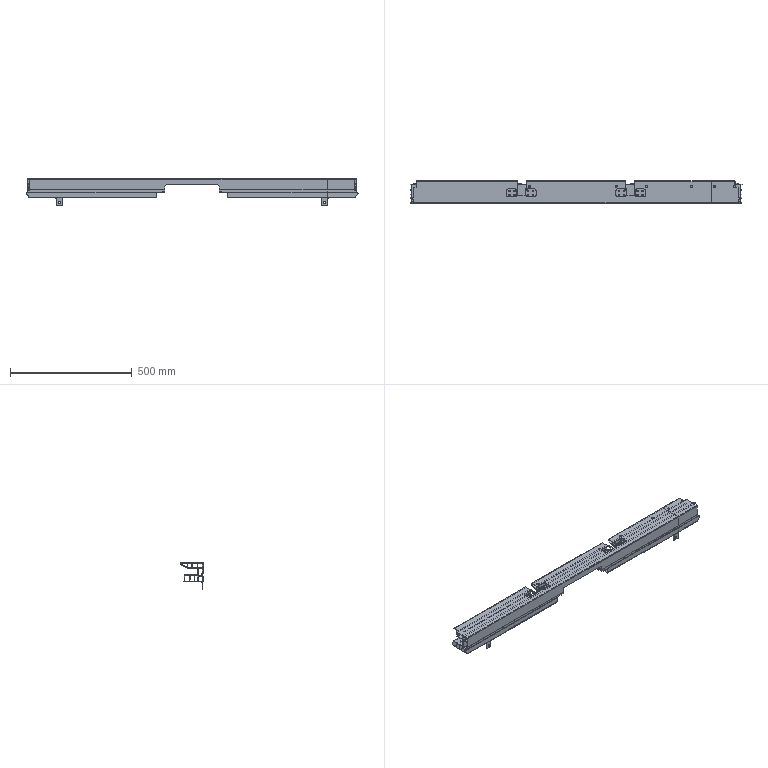NC program | NX | posted with a generic post | part box 1365 x 90.95 x 108.501 mm
Lines 6615 to 7500 of 25066:
(CAVITY_MILL_COPY , TOOL : D10)
N13216 T10 M6
N13218 G54
N13220 G17 G0 G90 X-676.615 Y32.745 B0. C0. S6500 M3
N13222 G43 Z30. H10
N13224 Z0.508
N13226 G94 G1 Z-0.992 F1000.
N13228 X-675.092 Y31.92
N13230 G3 X-674.092 Y31.947 R1.
N13232 G1 X-672.75 Y32.772 F1800.
N13234 Y34.347
N13236 G3 X-673.25 Y35.213 R1.
N13238 G1 X-674.75 Y36.079
N13240 Z0.508
N13242 G0 X-676.615 Y32.745 Z-0.482
N13244 G1 Z-1.982 F1000.
N13246 X-675.092 Y31.92
N13248 G3 X-674.092 Y31.947 R1.
N13250 G1 X-672.75 Y32.772 F1800.
N13252 Y34.347
N13254 G3 X-673.25 Y35.213 R1.
N13256 G1 X-674.75 Y36.079
N13258 Z-0.482
N13260 G0 X-676.615 Y32.745 Z-1.473
N13262 G1 Z-2.973 F1000.
N13264 X-675.092 Y31.92
N13266 G3 X-674.092 Y31.947 R1.
N13268 G1 X-672.75 Y32.772 F1800.
N13270 Y34.347
N13272 G3 X-673.25 Y35.213 R1.
N13274 G1 X-674.75 Y36.079
N13276 Z-1.473
N13278 G0 X-676.615 Y32.745 Z-2.463
N13280 G1 Z-3.963 F1000.
N13282 X-675.092 Y31.92
N13284 G3 X-674.092 Y31.947 R1.
N13286 G1 X-672.75 Y32.772 F1800.
N13288 Y34.347
N13290 G3 X-673.25 Y35.213 R1.
N13292 G1 X-674.75 Y36.079
N13294 Z-2.463
N13296 G0 X-676.615 Y32.745 Z-3.454
N13298 G1 Z-4.954 F1000.
N13300 X-675.092 Y31.92
N13302 G3 X-674.092 Y31.947 R1.
N13304 G1 X-672.75 Y32.772 F1800.
N13306 Y34.347
N13308 G3 X-673.25 Y35.213 R1.
N13310 G1 X-674.75 Y36.079
N13312 Z-3.454
N13314 G0 X-676.615 Y32.745 Z-4.444
N13316 G1 Z-5.944 F1000.
N13318 X-675.092 Y31.92
N13320 G3 X-674.092 Y31.947 R1.
N13322 G1 X-672.75 Y32.772 F1800.
N13324 Y34.347
N13326 G3 X-673.25 Y35.213 R1.
N13328 G1 X-674.75 Y36.079
N13330 Z-4.444
N13332 G0 X-676.615 Y32.745 Z-5.435
N13334 G1 Z-6.935 F1000.
N13336 X-675.092 Y31.92
N13338 G3 X-674.092 Y31.947 R1.
N13340 G1 X-672.75 Y32.772 F1800.
N13342 Y34.347
N13344 G3 X-673.25 Y35.213 R1.
N13346 G1 X-674.75 Y36.079
N13348 Z-5.435
N13350 G0 X-676.615 Y32.745 Z-6.425
N13352 G1 Z-7.925 F1000.
N13354 X-675.092 Y31.92
N13356 G3 X-674.092 Y31.947 R1.
N13358 G1 X-672.75 Y32.772 F1800.
N13360 Y34.347
N13362 G3 X-673.25 Y35.213 R1.
N13364 G1 X-674.75 Y36.079
N13366 Z-6.425
N13368 G0 X-676.615 Y32.745 Z-7.416
N13370 G1 Z-8.916 F1000.
N13372 X-675.092 Y31.92
N13374 G3 X-674.092 Y31.947 R1.
N13376 G1 X-672.75 Y32.772 F1800.
N13378 Y34.347
N13380 G3 X-673.25 Y35.213 R1.
N13382 G1 X-674.75 Y36.079
N13384 Z-7.416
N13386 G0 X-676.615 Y32.745 Z-8.406
N13388 G1 Z-9.906 F1000.
N13390 X-675.092 Y31.92
N13392 G3 X-674.092 Y31.947 R1.
N13394 G1 X-672.75 Y32.772 F1800.
N13396 Y34.347
N13398 G3 X-673.25 Y35.213 R1.
N13400 G1 X-674.75 Y36.079
N13402 Z-8.406
N13404 G0 X-676.615 Y32.745 Z-9.397
N13406 G1 Z-10.897 F1000.
N13408 X-675.092 Y31.92
N13410 G3 X-674.092 Y31.947 R1.
N13412 G1 X-672.75 Y32.772 F1800.
N13414 Y34.347
N13416 G3 X-673.25 Y35.213 R1.
N13418 G1 X-674.75 Y36.079
N13420 Z-9.397
N13422 G0 X-676.615 Y32.745 Z-10.387
N13424 G1 Z-11.887 F1000.
N13426 X-675.092 Y31.92
N13428 G3 X-674.092 Y31.947 R1.
N13430 G1 X-672.75 Y32.772 F1800.
N13432 Y34.347
N13434 G3 X-673.25 Y35.213 R1.
N13436 G1 X-674.75 Y36.079
N13438 Z-10.387
N13440 G0 X-676.615 Y32.745 Z-11.377
N13442 G1 Z-12.877 F1000.
N13444 X-675.092 Y31.92
N13446 G3 X-674.092 Y31.947 R1.
N13448 G1 X-672.75 Y32.772 F1800.
N13450 Y34.347
N13452 G3 X-673.25 Y35.213 R1.
N13454 G1 X-674.75 Y36.079
N13456 Z-11.377
N13458 G0 X-676.615 Y32.745 Z-12.368
N13460 G1 Z-13.868 F1000.
N13462 X-675.092 Y31.92
N13464 G3 X-674.092 Y31.947 R1.
N13466 G1 X-672.75 Y32.772 F1800.
N13468 Y34.347
N13470 G3 X-673.25 Y35.213 R1.
N13472 G1 X-674.75 Y36.079
N13474 Z-12.368
N13476 G0 X-676.615 Y32.745 Z-13.358
N13478 G1 Z-14.858 F1000.
N13480 X-675.092 Y31.92
N13482 G3 X-674.092 Y31.947 R1.
N13484 G1 X-672.75 Y32.772 F1800.
N13486 Y34.347
N13488 G3 X-673.25 Y35.213 R1.
N13490 G1 X-674.75 Y36.079
N13492 Z-13.358
N13494 G0 X-676.615 Y32.745 Z-14.349
N13496 G1 Z-15.849 F1000.
N13498 X-675.092 Y31.92
N13500 G3 X-674.092 Y31.947 R1.
N13502 G1 X-672.75 Y32.772 F1800.
N13504 Y34.347
N13506 G3 X-673.25 Y35.213 R1.
N13508 G1 X-674.75 Y36.079
N13510 Z-14.349
N13512 G0 X-676.615 Y32.745 Z-15.339
N13514 G1 Z-16.839 F1000.
N13516 X-675.092 Y31.92
N13518 G3 X-674.092 Y31.947 R1.
N13520 G1 X-672.75 Y32.772 F1800.
N13522 Y34.347
N13524 G3 X-673.25 Y35.213 R1.
N13526 G1 X-674.75 Y36.079
N13528 Z-15.339
N13530 G0 X-676.615 Y32.745 Z-16.33
N13532 G1 Z-17.83 F1000.
N13534 X-675.092 Y31.92
N13536 G3 X-674.092 Y31.947 R1.
N13538 G1 X-672.75 Y32.772 F1800.
N13540 Y34.347
N13542 G3 X-673.25 Y35.213 R1.
N13544 G1 X-674.75 Y36.079
N13546 Z-16.33
N13548 G0 X-676.615 Y32.745 Z-17.32
N13550 G1 Z-18.82 F1000.
N13552 X-675.092 Y31.92
N13554 G3 X-674.092 Y31.947 R1.
N13556 G1 X-672.75 Y32.772 F1800.
N13558 Y34.347
N13560 G3 X-673.25 Y35.213 R1.
N13562 G1 X-674.75 Y36.079
N13564 Z-17.32
N13566 G0 X-676.615 Y32.745 Z-18.311
N13568 G1 Z-19.811 F1000.
N13570 X-675.092 Y31.92
N13572 G3 X-674.092 Y31.947 R1.
N13574 G1 X-672.75 Y32.772 F1800.
N13576 Y34.347
N13578 G3 X-673.25 Y35.213 R1.
N13580 G1 X-674.75 Y36.079
N13582 Z-18.311
N13584 G0 X-676.615 Y32.745 Z-19.301
N13586 G1 Z-20.801 F1000.
N13588 X-675.092 Y31.92
N13590 G3 X-674.092 Y31.947 R1.
N13592 G1 X-672.75 Y32.772 F1800.
N13594 Y34.347
N13596 G3 X-673.25 Y35.213 R1.
N13598 G1 X-674.75 Y36.079
N13600 Z-19.301
N13602 G0 X-676.615 Y32.745 Z-20.291
N13604 G1 Z-21.791 F1000.
N13606 X-675.092 Y31.92
N13608 G3 X-674.092 Y31.947 R1.
N13610 G1 X-672.75 Y32.772 F1800.
N13612 Y34.347
N13614 G3 X-673.25 Y35.213 R1.
N13616 G1 X-674.75 Y36.079
N13618 Z-20.291
N13620 G0 X-676.615 Y32.745 Z-21.28
N13622 G1 Z-22.78 F1000.
N13624 X-675.092 Y31.92
N13626 G3 X-674.092 Y31.947 R1.
N13628 G1 X-672.75 Y32.772 F1800.
N13630 Y34.347
N13632 G3 X-673.25 Y35.213 R1.
N13634 G1 X-674.75 Y36.079
N13636 Z-21.28
N13638 G0 X-676.615 Y32.745 Z-22.269
N13640 G1 Z-23.769 F1000.
N13642 X-675.092 Y31.92
N13644 G3 X-674.092 Y31.947 R1.
N13646 G1 X-672.75 Y32.772 F1800.
N13648 Y34.347
N13650 G3 X-673.25 Y35.213 R1.
N13652 G1 X-674.75 Y36.079
N13654 Z-22.269
N13656 G0 X-676.615 Y32.745 Z-23.258
N13658 G1 Z-24.758 F1000.
N13660 X-675.092 Y31.92
N13662 G3 X-674.092 Y31.947 R1.
N13664 G1 X-672.75 Y32.772 F1800.
N13666 Y34.347
N13668 G3 X-673.25 Y35.213 R1.
N13670 G1 X-674.75 Y36.079
N13672 Z-23.258
N13674 G0 X-676.615 Y32.745 Z-24.248
N13676 G1 Z-25.748 F1000.
N13678 X-675.092 Y31.92
N13680 G3 X-674.092 Y31.947 R1.
N13682 G1 X-672.75 Y32.772 F1800.
N13684 Y34.347
N13686 G3 X-673.25 Y35.213 R1.
N13688 G1 X-674.75 Y36.079
N13690 Z-24.248
N13692 G0 X-676.615 Y32.745 Z-25.237
N13694 G1 Z-26.737 F1000.
N13696 X-675.092 Y31.92
N13698 G3 X-674.092 Y31.947 R1.
N13700 G1 X-672.75 Y32.772 F1800.
N13702 Y34.347
N13704 G3 X-673.25 Y35.213 R1.
N13706 G1 X-674.75 Y36.079
N13708 Z-25.237
N13710 G0 X-676.615 Y32.745 Z-26.226
N13712 G1 Z-27.726 F1000.
N13714 X-675.092 Y31.92
N13716 G3 X-674.092 Y31.947 R1.
N13718 G1 X-672.75 Y32.772 F1800.
N13720 Y34.347
N13722 G3 X-673.25 Y35.213 R1.
N13724 G1 X-674.75 Y36.079
N13726 Z-26.226
N13728 G0 X-676.615 Y32.745 Z-27.216
N13730 G1 Z-28.716 F1000.
N13732 X-675.092 Y31.92
N13734 G3 X-674.092 Y31.947 R1.
N13736 G1 X-672.75 Y32.772 F1800.
N13738 Y34.347
N13740 G3 X-673.25 Y35.213 R1.
N13742 G1 X-674.75 Y36.079
N13744 Z-27.216
N13746 G0 X-676.615 Y32.745 Z-28.205
N13748 G1 Z-29.705 F1000.
N13750 X-675.092 Y31.92
N13752 G3 X-674.092 Y31.947 R1.
N13754 G1 X-672.75 Y32.772 F1800.
N13756 Y34.347
N13758 G3 X-673.25 Y35.213 R1.
N13760 G1 X-674.75 Y36.079
N13762 Z-28.205
N13764 G0 X-676.615 Y32.745 Z-29.194
N13766 G1 Z-30.694 F1000.
N13768 X-675.092 Y31.92
N13770 G3 X-674.092 Y31.947 R1.
N13772 G1 X-672.75 Y32.772 F1800.
N13774 Y34.347
N13776 G3 X-673.25 Y35.213 R1.
N13778 G1 X-674.75 Y36.079
N13780 Z-29.194
N13782 G0 X-676.615 Y32.745 Z-30.183
N13784 G1 Z-31.683 F1000.
N13786 X-675.092 Y31.92
N13788 G3 X-674.092 Y31.947 R1.
N13790 G1 X-672.75 Y32.772 F1800.
N13792 Y34.347
N13794 G3 X-673.25 Y35.213 R1.
N13796 G1 X-674.75 Y36.079
N13798 Z-30.183
N13800 G0 X-676.615 Y32.745 Z-31.173
N13802 G1 Z-32.673 F1000.
N13804 X-675.092 Y31.92
N13806 G3 X-674.092 Y31.947 R1.
N13808 G1 X-672.75 Y32.772 F1800.
N13810 Y34.347
N13812 G3 X-673.25 Y35.213 R1.
N13814 G1 X-674.75 Y36.079
N13816 Z-31.173
N13818 G0 X-676.615 Y32.745 Z-32.162
N13820 G1 Z-33.662 F1000.
N13822 X-675.092 Y31.92
N13824 G3 X-674.092 Y31.947 R1.
N13826 G1 X-672.75 Y32.772 F1800.
N13828 Y34.347
N13830 G3 X-673.25 Y35.213 R1.
N13832 G1 X-674.75 Y36.079
N13834 Z-32.162
N13836 G0 X-676.615 Y32.745 Z-33.151
N13838 G1 Z-34.651 F1000.
N13840 X-675.092 Y31.92
N13842 G3 X-674.092 Y31.947 R1.
N13844 G1 X-672.75 Y32.772 F1800.
N13846 Y34.347
N13848 G3 X-673.25 Y35.213 R1.
N13850 G1 X-674.75 Y36.079
N13852 Z-33.151
N13854 G0 X-676.615 Y32.745 Z-34.141
N13856 G1 Z-35.641 F1000.
N13858 X-675.092 Y31.92
N13860 G3 X-674.092 Y31.947 R1.
N13862 G1 X-672.75 Y32.772 F1800.
N13864 Y34.347
N13866 G3 X-673.25 Y35.213 R1.
N13868 G1 X-674.75 Y36.079
N13870 Z-34.141
N13872 G0 X-676.615 Y32.745 Z-35.13
N13874 G1 Z-36.63 F1000.
N13876 X-675.092 Y31.92
N13878 G3 X-674.092 Y31.947 R1.
N13880 G1 X-672.75 Y32.772 F1800.
N13882 Y34.347
N13884 G3 X-673.25 Y35.213 R1.
N13886 G1 X-674.75 Y36.079
N13888 Z-35.13
N13890 G0 X-676.615 Y32.745 Z-36.119
N13892 G1 Z-37.619 F1000.
N13894 X-675.092 Y31.92
N13896 G3 X-674.092 Y31.947 R1.
N13898 G1 X-672.75 Y32.772 F1800.
N13900 Y34.347
N13902 G3 X-673.25 Y35.213 R1.
N13904 G1 X-674.75 Y36.079
N13906 Z-36.119
N13908 G0 X-676.615 Y32.745 Z-37.108
N13910 G1 Z-38.608 F1000.
N13912 X-675.092 Y31.92
N13914 G3 X-674.092 Y31.947 R1.
N13916 G1 X-672.75 Y32.772 F1800.
N13918 Y34.347
N13920 G3 X-673.25 Y35.213 R1.
N13922 G1 X-674.75 Y36.079
N13924 Z-37.108
N13926 G0 X-676.615 Y32.745 Z-38.098
N13928 G1 Z-39.598 F1000.
N13930 X-675.092 Y31.92
N13932 G3 X-674.092 Y31.947 R1.
N13934 G1 X-672.75 Y32.772 F1800.
N13936 Y34.347
N13938 G3 X-673.25 Y35.213 R1.
N13940 G1 X-674.75 Y36.079
N13942 Z-38.098
N13944 G0 X-676.615 Y32.745 Z-39.087
N13946 G1 Z-40.587 F1000.
N13948 X-675.092 Y31.92
N13950 G3 X-674.092 Y31.947 R1.
N13952 G1 X-672.75 Y32.772 F1800.
N13954 Y34.347
N13956 G3 X-673.25 Y35.213 R1.
N13958 G1 X-674.75 Y36.079
N13960 Z-39.087
N13962 G0 X-676.615 Y32.745 Z-40.076
N13964 G1 Z-41.576 F1000.
N13966 X-675.092 Y31.92
N13968 G3 X-674.092 Y31.947 R1.
N13970 G1 X-672.75 Y32.772 F1800.
N13972 Y34.347
N13974 G3 X-673.25 Y35.213 R1.
N13976 G1 X-674.75 Y36.079
N13978 Z-40.076
N13980 G0 X-676.615 Y32.745 Z-41.066
N13982 G1 Z-42.566 F1000.
N13984 X-675.092 Y31.92
N13986 G3 X-674.092 Y31.947 R1.
N13988 G1 X-672.75 Y32.772 F1800.
N13990 Y34.347
N13992 G3 X-673.25 Y35.213 R1.
N13994 G1 X-674.75 Y36.079
N13996 Z-41.066
N13998 G0 X-676.615 Y32.745 Z-42.055
N14000 G1 Z-43.555 F1000.
N14002 X-675.092 Y31.92
N14004 G3 X-674.092 Y31.947 R1.
N14006 G1 X-672.75 Y32.772 F1800.
N14008 Y34.347
N14010 G3 X-673.25 Y35.213 R1.
N14012 G1 X-674.75 Y36.079
N14014 Z-42.055
N14016 G0 X-676.615 Y32.745 Z-43.044
N14018 G1 Z-44.544 F1000.
N14020 X-675.092 Y31.92
N14022 G3 X-674.092 Y31.947 R1.
N14024 G1 X-672.75 Y32.772 F1800.
N14026 Y34.347
N14028 G3 X-673.25 Y35.213 R1.
N14030 G1 X-674.75 Y36.079
N14032 Z-43.044
N14034 G0 X-676.615 Y32.745 Z-44.033
N14036 G1 Z-45.533 F1000.
N14038 X-675.092 Y31.92
N14040 G3 X-674.092 Y31.947 R1.
N14042 G1 X-672.75 Y32.772 F1800.
N14044 Y34.347
N14046 G3 X-673.25 Y35.213 R1.
N14048 G1 X-674.75 Y36.079
N14050 Z-44.033
N14052 G0 X-676.615 Y32.745 Z-45.023
N14054 G1 Z-46.523 F1000.
N14056 X-675.092 Y31.92
N14058 G3 X-674.092 Y31.947 R1.
N14060 G1 X-672.75 Y32.772 F1800.
N14062 Y34.347
N14064 G3 X-673.25 Y35.213 R1.
N14066 G1 X-674.75 Y36.079
N14068 Z-45.023
N14070 G0 X-676.615 Y32.745 Z-46.012
N14072 G1 Z-47.512 F1000.
N14074 X-675.092 Y31.92
N14076 G3 X-674.092 Y31.947 R1.
N14078 G1 X-672.75 Y32.772 F1800.
N14080 Y34.347
N14082 G3 X-673. Y34.78 R0.5
N14084 G1 X-675.764 Y36.376
N14086 Z-46.012
N14088 G0 Z30.
N14090 X-674.75 Y34.437
N14092 Z-45.023
N14094 G1 Z-46.523 F1000.
N14096 X-673.25 Y35.303
N14098 G3 X-672.75 Y36.169 R1.
N14100 G1 Y36.947 F1800.
N14102 G2 X-673.144 Y37.537 R4.848
N14104 G3 X-674.005 Y38.045 R1.
N14106 G1 X-675.513 Y38.059
N14108 Z-45.023
N14110 G0 X-679.821 Y30.125 Z-46.012
N14112 G1 Z-47.512 F1000.
N14114 X-673.25 Y33.918
N14116 G3 X-672.75 Y34.784 R1.
N14118 G1 Y35.967 F1800.
N14120 G2 X-673.506 Y36.662 R5.001
N14122 G3 X-674.454 Y36.98 R1.
N14124 G1 X-675.936 Y36.679
N14126 Z-46.012
N14128 G0 X-677.106 Y32.443 Z-47.001
N14130 G1 Z-48.501 F1000.
N14132 X-675.583 Y31.618
N14134 G3 X-674.584 Y31.645 R1.
N14136 G1 X-672.75 Y32.772 F1800.
N14138 Y35.396
N14140 G2 X-674.232 Y36.397 R5.012
N14142 G3 X-675.201 Y36.644 R1.
N14144 G1 X-676.657 Y36.236
N14146 Z-47.001
N14148 G0 Z30.
N14150 X-675.481 Y44.484
N14152 Z-45.023
N14154 G1 Z-46.523 F1000.
N14156 X-673.971 Y44.479
N14158 G3 X-673.104 Y44.976 R1.
N14160 G2 X-672.75 Y45.504 R4.926 F1800.
N14162 X-672.706 Y46.141 R5.
N14164 G3 X-673.086 Y47.065 R1.
N14166 G1 X-674.283 Y47.989
N14168 Z-45.023
N14170 G0 X-675.606 Y46.327 Z-46.012
N14172 G1 Z-47.512 F1000.
N14174 X-674.156 Y45.895
N14176 G3 X-673.183 Y46.126 R1.
N14178 G2 X-672.626 Y46.582 R5.042 F1800.
N14180 X-672.415 Y47.274 R5.
N14182 G3 X-672.57 Y48.261 R1.
N14184 G1 X-673.52 Y49.438
N14186 Z-46.012
N14188 G0 X-675.405 Y47.697 Z-47.001
N14190 G1 Z-48.501 F1000.
N14192 X-673.879 Y46.994
N14194 G3 X-672.883 Y47.085 R1.
N14196 G1 X-672.333 Y47.474 F1800.
N14198 G2 X-672.032 Y48.057 R5.
N14200 G3 X-672.013 Y49.057 R1.
N14202 G1 X-672.744 Y50.381
N14204 Z-47.001
N14206 G0 Z30.
N14208 X-674.75 Y11.607
N14210 Z0.508
N14212 G1 Z-0.992 F1000.
N14214 X-673.25 Y12.473
N14216 G3 X-672.75 Y13.339 R1.
N14218 G1 Y15.775 F1800.
N14220 G2 X-674.846 Y16.096 R7.
N14222 G3 X-675.822 Y15.878 R1.
N14224 G1 X-676.968 Y14.825
N14226 Z0.508
N14228 G0 X-674.75 Y11.607 Z-0.482
N14230 G1 Z-1.982 F1000.
N14232 X-673.25 Y12.473
N14234 G3 X-672.75 Y13.339 R1.
N14236 G1 Y15.775 F1800.
N14238 G2 X-674.846 Y16.096 R7.
N14240 G3 X-675.822 Y15.878 R1.
N14242 G1 X-676.968 Y14.825
N14244 Z-0.482
N14246 G0 X-674.75 Y11.607 Z-1.473
N14248 G1 Z-2.973 F1000.
N14250 X-673.25 Y12.473
N14252 G3 X-672.75 Y13.339 R1.
N14254 G1 Y15.775 F1800.
N14256 G2 X-674.846 Y16.096 R7.
N14258 G3 X-675.822 Y15.878 R1.
N14260 G1 X-676.968 Y14.825
N14262 Z-1.473
N14264 G0 X-674.75 Y11.607 Z-2.463
N14266 G1 Z-3.963 F1000.
N14268 X-673.25 Y12.473
N14270 G3 X-672.75 Y13.339 R1.
N14272 G1 Y15.775 F1800.
N14274 G2 X-674.846 Y16.096 R7.
N14276 G3 X-675.822 Y15.878 R1.
N14278 G1 X-676.968 Y14.825
N14280 Z-2.463
N14282 G0 X-674.75 Y11.607 Z-3.454
N14284 G1 Z-4.954 F1000.
N14286 X-673.25 Y12.473
N14288 G3 X-672.75 Y13.339 R1.
N14290 G1 Y15.775 F1800.
N14292 G2 X-674.846 Y16.096 R7.
N14294 G3 X-675.822 Y15.878 R1.
N14296 G1 X-676.968 Y14.825
N14298 Z-3.454
N14300 G0 X-674.75 Y11.607 Z-4.444
N14302 G1 Z-5.944 F1000.
N14304 X-673.25 Y12.473
N14306 G3 X-672.75 Y13.339 R1.
N14308 G1 Y15.775 F1800.
N14310 G2 X-674.846 Y16.096 R7.
N14312 G3 X-675.822 Y15.878 R1.
N14314 G1 X-676.968 Y14.825
N14316 Z-4.444
N14318 G0 X-674.75 Y11.607 Z-5.435
N14320 G1 Z-6.935 F1000.
N14322 X-673.25 Y12.473
N14324 G3 X-672.75 Y13.339 R1.
N14326 G1 Y15.775 F1800.
N14328 G2 X-674.846 Y16.096 R7.
N14330 G3 X-675.822 Y15.878 R1.
N14332 G1 X-676.968 Y14.825
N14334 Z-5.435
N14336 G0 X-674.75 Y11.607 Z-6.425
N14338 G1 Z-7.925 F1000.
N14340 X-673.25 Y12.473
N14342 G3 X-672.75 Y13.339 R1.
N14344 G1 Y15.775 F1800.
N14346 G2 X-674.846 Y16.096 R7.
N14348 G3 X-675.822 Y15.878 R1.
N14350 G1 X-676.968 Y14.825
N14352 Z-6.425
N14354 G0 X-674.75 Y11.607 Z-7.416
N14356 G1 Z-8.916 F1000.
N14358 X-673.25 Y12.473
N14360 G3 X-672.75 Y13.339 R1.
N14362 G1 Y15.775 F1800.
N14364 G2 X-674.846 Y16.096 R7.
N14366 G3 X-675.822 Y15.878 R1.
N14368 G1 X-676.968 Y14.825
N14370 Z-7.416
N14372 G0 X-674.75 Y11.607 Z-8.406
N14374 G1 Z-9.906 F1000.
N14376 X-673.25 Y12.473
N14378 G3 X-672.75 Y13.339 R1.
N14380 G1 Y15.775 F1800.
N14382 G2 X-674.846 Y16.096 R7.
N14384 G3 X-675.822 Y15.878 R1.
N14386 G1 X-676.968 Y14.825
N14388 Z-8.406
N14390 G0 X-674.75 Y11.607 Z-9.397
N14392 G1 Z-10.897 F1000.
N14394 X-673.25 Y12.473
N14396 G3 X-672.75 Y13.339 R1.
N14398 G1 Y15.775 F1800.
N14400 G2 X-674.846 Y16.096 R7.
N14402 G3 X-675.822 Y15.878 R1.
N14404 G1 X-676.968 Y14.825
N14406 Z-9.397
N14408 G0 X-674.75 Y11.607 Z-10.387
N14410 G1 Z-11.887 F1000.
N14412 X-673.25 Y12.473
N14414 G3 X-672.75 Y13.339 R1.
N14416 G1 Y15.775 F1800.
N14418 G2 X-674.846 Y16.096 R7.
N14420 G3 X-675.822 Y15.878 R1.
N14422 G1 X-676.968 Y14.825
N14424 Z-10.387
N14426 G0 X-674.75 Y11.607 Z-11.377
N14428 G1 Z-12.877 F1000.
N14430 X-673.25 Y12.473
N14432 G3 X-672.75 Y13.339 R1.
N14434 G1 Y15.775 F1800.
N14436 G2 X-674.846 Y16.096 R7.
N14438 G3 X-675.822 Y15.878 R1.
N14440 G1 X-676.968 Y14.825
N14442 Z-11.377
N14444 G0 X-674.75 Y11.607 Z-12.368
N14446 G1 Z-13.868 F1000.
N14448 X-673.25 Y12.473
N14450 G3 X-672.75 Y13.339 R1.
N14452 G1 Y15.775 F1800.
N14454 G2 X-674.846 Y16.096 R7.
N14456 G3 X-675.822 Y15.878 R1.
N14458 G1 X-676.968 Y14.825
N14460 Z-12.368
N14462 G0 X-674.75 Y11.607 Z-13.358
N14464 G1 Z-14.858 F1000.
N14466 X-673.25 Y12.473
N14468 G3 X-672.75 Y13.339 R1.
N14470 G1 Y15.775 F1800.
N14472 G2 X-674.846 Y16.096 R7.
N14474 G3 X-675.822 Y15.878 R1.
N14476 G1 X-676.968 Y14.825
N14478 Z-13.358
N14480 G0 X-674.75 Y11.607 Z-14.349
N14482 G1 Z-15.849 F1000.
N14484 X-673.25 Y12.473
N14486 G3 X-672.75 Y13.339 R1.
N14488 G1 Y15.775 F1800.
N14490 G2 X-674.846 Y16.096 R7.
N14492 G3 X-675.822 Y15.878 R1.
N14494 G1 X-676.968 Y14.825
N14496 Z-14.349
N14498 G0 X-674.75 Y11.607 Z-15.339
N14500 G1 Z-16.839 F1000.
N14502 X-673.25 Y12.473
N14504 G3 X-672.75 Y13.339 R1.
N14506 G1 Y15.775 F1800.
N14508 G2 X-674.846 Y16.096 R7.
N14510 G3 X-675.822 Y15.878 R1.
N14512 G1 X-676.968 Y14.825
N14514 Z-15.339
N14516 G0 X-674.75 Y11.607 Z-16.33
N14518 G1 Z-17.83 F1000.
N14520 X-673.25 Y12.473
N14522 G3 X-672.75 Y13.339 R1.
N14524 G1 Y15.775 F1800.
N14526 G2 X-674.846 Y16.096 R7.
N14528 G3 X-675.822 Y15.878 R1.
N14530 G1 X-676.968 Y14.825
N14532 Z-16.33
N14534 G0 X-674.75 Y11.607 Z-17.32
N14536 G1 Z-18.82 F1000.
N14538 X-673.25 Y12.473
N14540 G3 X-672.75 Y13.339 R1.
N14542 G1 Y15.775 F1800.
N14544 G2 X-674.846 Y16.096 R7.
N14546 G3 X-675.822 Y15.878 R1.
N14548 G1 X-676.968 Y14.825
N14550 Z-17.32
N14552 G0 X-674.75 Y11.607 Z-18.311
N14554 G1 Z-19.811 F1000.
N14556 X-673.25 Y12.473
N14558 G3 X-672.75 Y13.339 R1.
N14560 G1 Y15.775 F1800.
N14562 G2 X-674.846 Y16.096 R7.
N14564 G3 X-675.822 Y15.878 R1.
N14566 G1 X-676.968 Y14.825
N14568 Z-18.311
N14570 G0 X-674.75 Y11.607 Z-19.301
N14572 G1 Z-20.801 F1000.
N14574 X-673.25 Y12.473
N14576 G3 X-672.75 Y13.339 R1.
N14578 G1 Y15.775 F1800.
N14580 G2 X-674.846 Y16.096 R7.
N14582 G3 X-675.822 Y15.878 R1.
N14584 G1 X-676.968 Y14.825
N14586 Z-19.301
N14588 G0 X-674.75 Y11.607 Z-20.291
N14590 G1 Z-21.791 F1000.
N14592 X-673.25 Y12.473
N14594 G3 X-672.75 Y13.339 R1.
N14596 G1 Y15.775 F1800.
N14598 G2 X-674.846 Y16.096 R7.
N14600 G3 X-675.822 Y15.878 R1.
N14602 G1 X-676.968 Y14.825
N14604 Z-20.291
N14606 G0 X-674.75 Y11.607 Z-21.28
N14608 G1 Z-22.78 F1000.
N14610 X-673.25 Y12.473
N14612 G3 X-672.75 Y13.339 R1.
N14614 G1 Y15.775 F1800.
N14616 G2 X-674.846 Y16.096 R7.
N14618 G3 X-675.822 Y15.878 R1.
N14620 G1 X-676.968 Y14.825
N14622 Z-21.28
N14624 G0 X-674.75 Y11.607 Z-22.269
N14626 G1 Z-23.769 F1000.
N14628 X-673.25 Y12.473
N14630 G3 X-672.75 Y13.339 R1.
N14632 G1 Y15.775 F1800.
N14634 G2 X-674.846 Y16.096 R7.
N14636 G3 X-675.822 Y15.878 R1.
N14638 G1 X-676.968 Y14.825
N14640 Z-22.269
N14642 G0 X-674.75 Y11.605 Z-23.258
N14644 G1 Z-24.758 F1000.
N14646 X-673.25 Y12.471
N14648 G3 X-672.75 Y13.337 R1.
N14650 G1 Y15.775 F1800.
N14652 G2 X-674.848 Y16.097 R7.
N14654 G3 X-675.825 Y15.88 R1.
N14656 G1 X-676.972 Y14.827
N14658 Z-23.258
N14660 G0 X-674.75 Y11.607 Z-24.248
N14662 G1 Z-25.748 F1000.
N14664 X-673.25 Y12.473
N14666 G3 X-672.75 Y13.339 R1.
N14668 G1 Y15.775 F1800.
N14670 G2 X-674.846 Y16.096 R7.
N14672 G3 X-675.822 Y15.878 R1.
N14674 G1 X-676.968 Y14.825
N14676 Z-24.248
N14678 G0 X-674.75 Y11.605 Z-25.237
N14680 G1 Z-26.737 F1000.
N14682 X-673.25 Y12.471
N14684 G3 X-672.75 Y13.337 R1.
N14686 G1 Y15.775 F1800.
N14688 G2 X-674.849 Y16.097 R7.
N14690 G3 X-675.825 Y15.88 R1.
N14692 G1 X-676.972 Y14.827
N14694 Z-25.237
N14696 G0 X-674.75 Y11.607 Z-26.226
N14698 G1 Z-27.726 F1000.
N14700 X-673.25 Y12.473
N14702 G3 X-672.75 Y13.339 R1.
N14704 G1 Y15.775 F1800.
N14706 G2 X-674.846 Y16.096 R7.
N14708 G3 X-675.822 Y15.878 R1.
N14710 G1 X-676.968 Y14.825
N14712 Z-26.226
N14714 G0 X-674.75 Y11.605 Z-27.216
N14716 G1 Z-28.716 F1000.
N14718 X-673.25 Y12.471
N14720 G3 X-672.75 Y13.337 R1.
N14722 G1 Y15.775 F1800.
N14724 G2 X-674.849 Y16.097 R7.
N14726 G3 X-675.825 Y15.88 R1.
N14728 G1 X-676.972 Y14.827
N14730 Z-27.216
N14732 G0 X-674.75 Y11.607 Z-28.205
N14734 G1 Z-29.705 F1000.
N14736 X-673.25 Y12.473
N14738 G3 X-672.75 Y13.339 R1.
N14740 G1 Y15.775 F1800.
N14742 G2 X-674.846 Y16.096 R7.
N14744 G3 X-675.822 Y15.878 R1.
N14746 G1 X-676.968 Y14.825
N14748 Z-28.205
N14750 G0 X-674.75 Y11.605 Z-29.194
N14752 G1 Z-30.694 F1000.
N14754 X-673.25 Y12.471
N14756 G3 X-672.75 Y13.337 R1.
N14758 G1 Y15.775 F1800.
N14760 G2 X-674.849 Y16.097 R7.
N14762 G3 X-675.825 Y15.88 R1.
N14764 G1 X-676.972 Y14.827
N14766 Z-29.194
N14768 G0 X-674.75 Y11.607 Z-30.183
N14770 G1 Z-31.683 F1000.
N14772 X-673.25 Y12.473
N14774 G3 X-672.75 Y13.339 R1.
N14776 G1 Y15.775 F1800.
N14778 G2 X-674.846 Y16.096 R7.
N14780 G3 X-675.822 Y15.878 R1.
N14782 G1 X-676.968 Y14.825
N14784 Z-30.183
N14786 G0 X-674.75 Y11.605 Z-31.173
N14788 G1 Z-32.673 F1000.
N14790 X-673.25 Y12.471
N14792 G3 X-672.75 Y13.337 R1.
N14794 G1 Y15.775 F1800.
N14796 G2 X-674.849 Y16.097 R7.
N14798 G3 X-675.825 Y15.88 R1.
N14800 G1 X-676.972 Y14.827
N14802 Z-31.173
N14804 G0 X-674.75 Y11.607 Z-32.162
N14806 G1 Z-33.662 F1000.
N14808 X-673.25 Y12.473
N14810 G3 X-672.75 Y13.339 R1.
N14812 G1 Y15.775 F1800.
N14814 G2 X-674.846 Y16.096 R7.
N14816 G3 X-675.822 Y15.878 R1.
N14818 G1 X-676.968 Y14.825
N14820 Z-32.162
N14822 G0 X-674.75 Y11.605 Z-33.151
N14824 G1 Z-34.651 F1000.
N14826 X-673.25 Y12.471
N14828 G3 X-672.75 Y13.337 R1.
N14830 G1 Y15.775 F1800.
N14832 G2 X-674.849 Y16.097 R7.
N14834 G3 X-675.825 Y15.88 R1.
N14836 G1 X-676.972 Y14.827
N14838 Z-33.151
N14840 G0 X-674.75 Y11.607 Z-34.141
N14842 G1 Z-35.641 F1000.
N14844 X-673.25 Y12.473
N14846 G3 X-672.75 Y13.339 R1.
N14848 G1 Y15.775 F1800.
N14850 G2 X-674.846 Y16.096 R7.
N14852 G3 X-675.822 Y15.878 R1.
N14854 G1 X-676.968 Y14.825
N14856 Z-34.141
N14858 G0 X-674.75 Y11.604 Z-35.13
N14860 G1 Z-36.63 F1000.
N14862 X-673.25 Y12.47
N14864 G3 X-672.75 Y13.336 R1.
N14866 G1 Y15.775 F1800.
N14868 G2 X-674.849 Y16.097 R7.
N14870 G3 X-675.825 Y15.88 R1.
N14872 G1 X-676.972 Y14.827
N14874 Z-35.13
N14876 G0 X-674.75 Y11.607 Z-36.119
N14878 G1 Z-37.619 F1000.
N14880 X-673.25 Y12.473
N14882 G3 X-672.75 Y13.339 R1.
N14884 G1 Y15.775 F1800.
N14886 G2 X-674.846 Y16.096 R7.
N14888 G3 X-675.822 Y15.878 R1.
N14890 G1 X-676.968 Y14.825
N14892 Z-36.119
N14894 G0 X-674.75 Y11.604 Z-37.108
N14896 G1 Z-38.608 F1000.
N14898 X-673.25 Y12.47
N14900 G3 X-672.75 Y13.336 R1.
N14902 G1 Y15.775 F1800.
N14904 G2 X-674.849 Y16.097 R7.
N14906 G3 X-675.825 Y15.88 R1.
N14908 G1 X-676.973 Y14.827
N14910 Z-37.108
N14912 G0 X-674.75 Y11.607 Z-38.098
N14914 G1 Z-39.598 F1000.
N14916 X-673.25 Y12.473
N14918 G3 X-672.75 Y13.339 R1.
N14920 G1 Y15.775 F1800.
N14922 G2 X-674.846 Y16.096 R7.
N14924 G3 X-675.822 Y15.878 R1.
N14926 G1 X-676.968 Y14.825
N14928 Z-38.098
N14930 G0 X-674.75 Y11.604 Z-39.087
N14932 G1 Z-40.587 F1000.
N14934 X-673.25 Y12.47
N14936 G3 X-672.75 Y13.336 R1.
N14938 G1 Y15.775 F1800.
N14940 G2 X-674.85 Y16.097 R7.
N14942 G3 X-675.826 Y15.88 R1.
N14944 G1 X-676.973 Y14.827
N14946 Z-39.087
N14948 G0 X-674.75 Y11.607 Z-40.076
N14950 G1 Z-41.576 F1000.
N14952 X-673.25 Y12.473
N14954 G3 X-672.75 Y13.339 R1.
N14956 G1 Y15.775 F1800.
N14958 G2 X-674.846 Y16.096 R7.
N14960 G3 X-675.822 Y15.878 R1.
N14962 G1 X-676.968 Y14.825
N14964 Z-40.076
N14966 G0 X-674.75 Y11.603 Z-41.066
N14968 G1 Z-42.566 F1000.
N14970 X-673.25 Y12.469
N14972 G3 X-672.75 Y13.335 R1.
N14974 G1 Y15.775 F1800.
N14976 G2 X-674.85 Y16.097 R7.
N14978 G3 X-675.826 Y15.88 R1.
N14980 G1 X-676.974 Y14.828